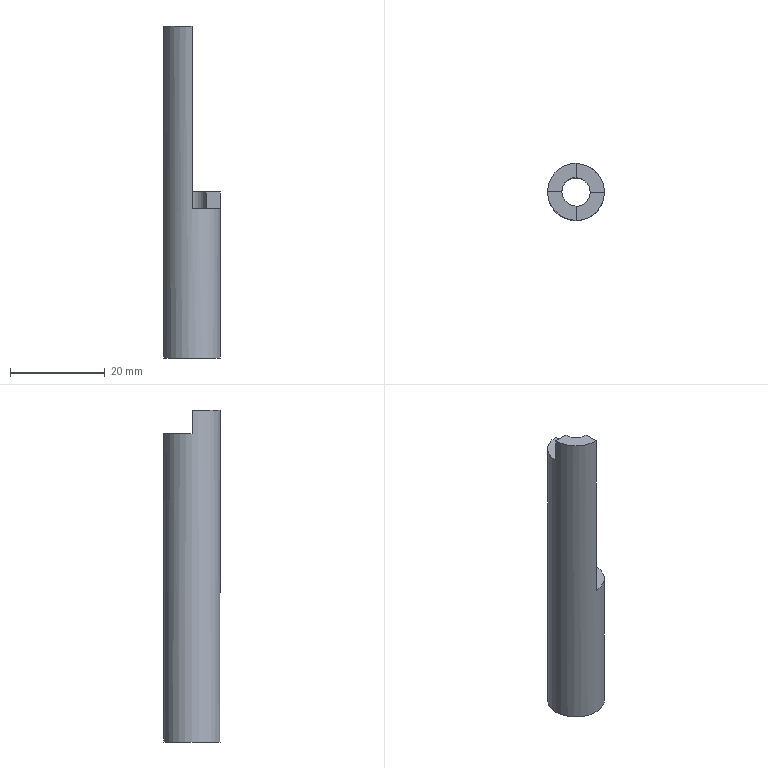Part | STEP file | SWF8-30_id742_x_t | 1 solid | 115 faces | box 12 x 12 x 70 mm | volume 4273 mm3 | plane 60 | other 53 | cylinder 2 | commonest cylinder face diameters 6 x1 12 x1